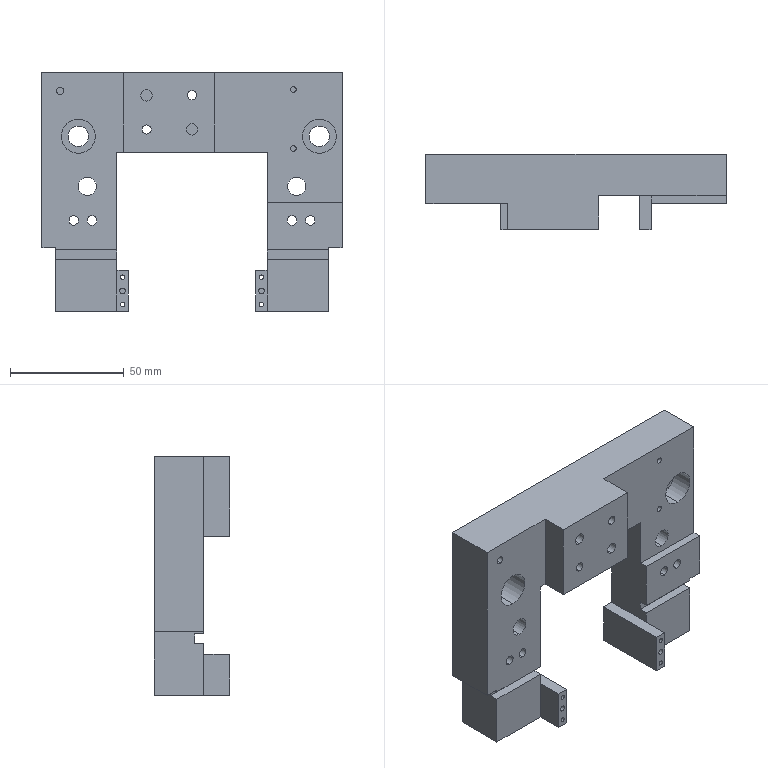Part | SolidWorks | features ICE 12, Extrusion 1 | 1 solid | 95 faces | box 132 x 33 x 105 mm | volume 188680 mm3 | plane 48 | cylinder 47 | commonest cylinder face diameters 2 x8 2.5 x8 4.2 x8 4 x4 5 x4 8 x4